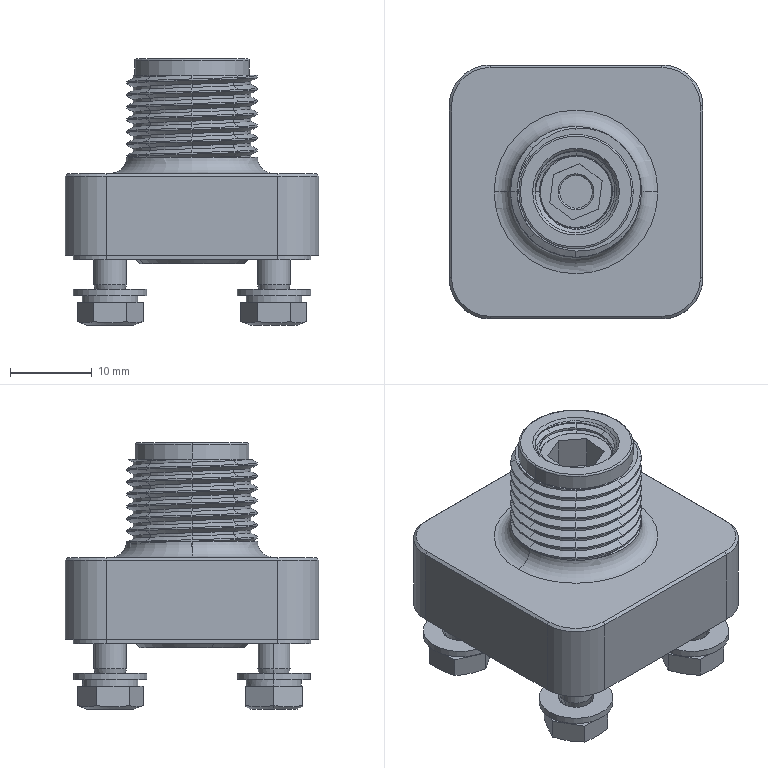Part | NX | features BREP 10 | 20 solids | 1867 faces | box 31 x 31 x 32.5 mm | volume 11689 mm3 | spline 898 | cylinder 675 | plane 211 | cone 67 | torus 16 | commonest cylinder face diameters 3.242 x212 4 x92 14.376 x66 11.376 x56 8.917 x53 8.817 x34